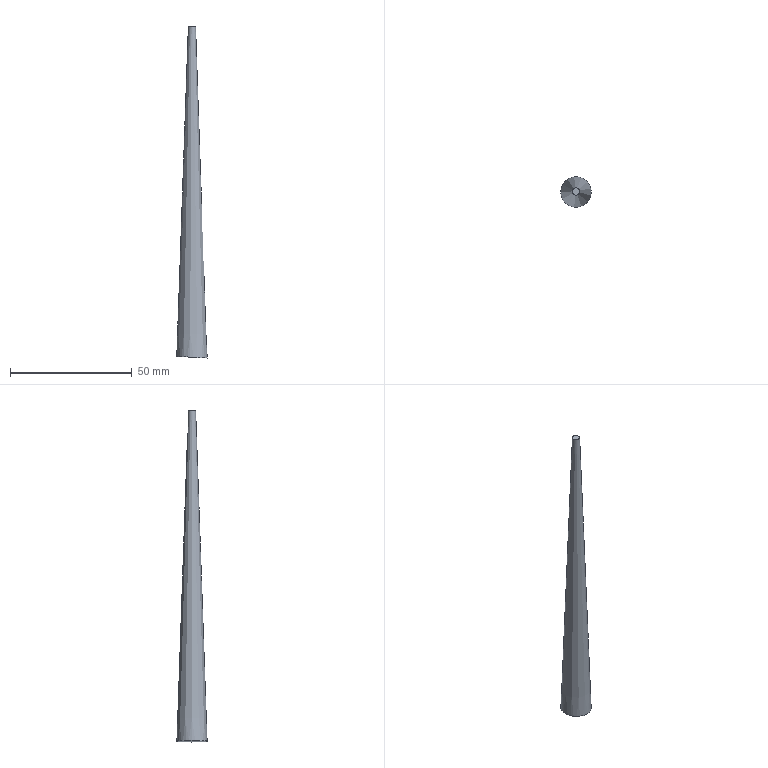Part | STEP file | solid 71 | 1 solid | 3 faces | box 12.511 x 12.511 x 136.502 mm | volume 7240 mm3 | plane 2 | cone 1